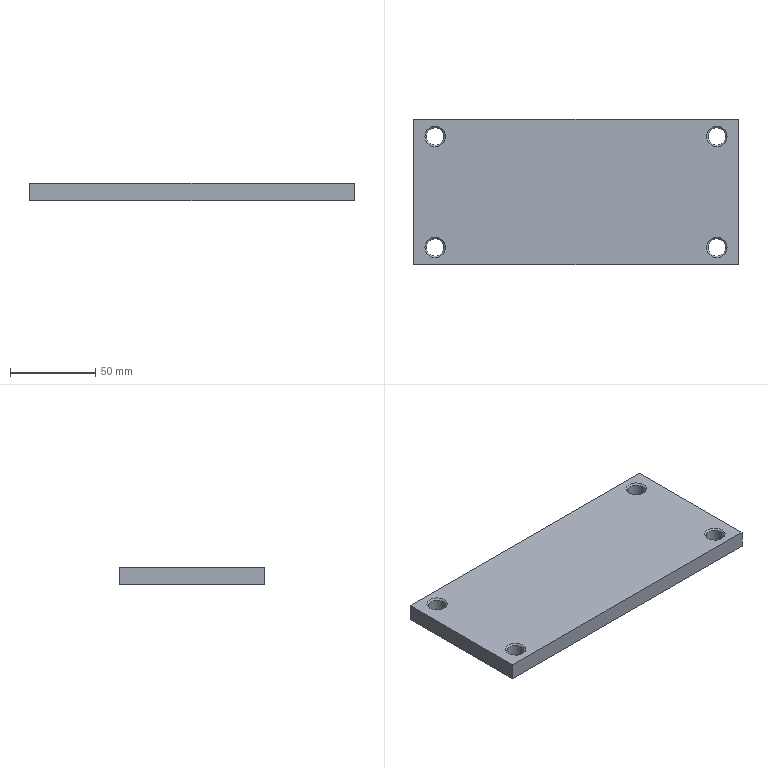Part | STEP file | Plate | 1 solid | 22 faces | box 190 x 85 x 10 mm | volume 158173 mm3 | cone 8 | cylinder 8 | plane 6 | commonest cylinder face diameters 10.2 x8
STEP:
#1=CARTESIAN_POINT('',(-147.6,57.5,9.075));
#2=VERTEX_POINT('',#1);
#3=CARTESIAN_POINT('',(-137.4,57.5,9.075));
#4=VERTEX_POINT('',#3);
#5=CARTESIAN_POINT('',(-142.5,57.5,9.075));
#6=DIRECTION('',(0.,0.,1.));
#7=DIRECTION('',(1.,0.,0.));
#8=AXIS2_PLACEMENT_3D('',#5,#6,#7);
#9=CIRCLE('',#8,5.1);
#10=EDGE_CURVE('',#2,#4,#9,.T.);
#11=ORIENTED_EDGE('',*,*,#10,.F.);
#12=CARTESIAN_POINT('',(-148.525,57.5,10.));
#13=VERTEX_POINT('',#12);
#14=CARTESIAN_POINT('',(-148.525,57.5,10.));
#15=DIRECTION('',(-0.7071,0.,0.7071));
#16=VECTOR('',#15,1000.);
#17=LINE('',#14,#16);
#18=EDGE_CURVE('',#2,#13,#17,.T.);
#19=ORIENTED_EDGE('',*,*,#18,.T.);
#20=CARTESIAN_POINT('',(-136.475,57.5,10.));
#21=VERTEX_POINT('',#20);
#22=CARTESIAN_POINT('',(-142.5,57.5,10.));
#23=DIRECTION('',(0.,0.,1.));
#24=DIRECTION('',(1.,0.,0.));
#25=AXIS2_PLACEMENT_3D('',#22,#23,#24);
#26=CIRCLE('',#25,6.025);
#27=EDGE_CURVE('',#13,#21,#26,.T.);
#28=ORIENTED_EDGE('',*,*,#27,.T.);
#29=CARTESIAN_POINT('',(-136.475,57.5,10.));
#30=DIRECTION('',(0.7071,0.,0.7071));
#31=VECTOR('',#30,1000.);
#32=LINE('',#29,#31);
#33=EDGE_CURVE('',#4,#21,#32,.T.);
#34=ORIENTED_EDGE('',*,*,#33,.F.);
#35=EDGE_LOOP('',(#11,#19,#28,#34));
#36=FACE_OUTER_BOUND('',#35,.T.);
#37=CARTESIAN_POINT('',(-142.5,57.5,10.));
#38=DIRECTION('',(0.,0.,1.));
#39=DIRECTION('',(1.,0.,0.));
#40=AXIS2_PLACEMENT_3D('',#37,#38,#39);
#41=CONICAL_SURFACE('',#40,6.025,0.7854);
#42=ADVANCED_FACE('',(#36),#41,.F.);
#43=CARTESIAN_POINT('',(-137.4,57.5,0.));
#44=VERTEX_POINT('',#43);
#45=CARTESIAN_POINT('',(-147.6,57.5,0.));
#46=VERTEX_POINT('',#45);
#47=CARTESIAN_POINT('',(-142.5,57.5,0.));
#48=DIRECTION('',(0.,0.,-1.));
#49=DIRECTION('',(-1.,0.,0.));
#50=AXIS2_PLACEMENT_3D('',#47,#48,#49);
#51=CIRCLE('',#50,5.1);
#52=EDGE_CURVE('',#44,#46,#51,.T.);
#53=ORIENTED_EDGE('',*,*,#52,.T.);
#54=CARTESIAN_POINT('',(-147.6,57.5,10.));
#55=DIRECTION('',(0.,0.,1.));
#56=VECTOR('',#55,1000.);
#57=LINE('',#54,#56);
#58=EDGE_CURVE('',#46,#2,#57,.T.);
#59=ORIENTED_EDGE('',*,*,#58,.T.);
#60=ORIENTED_EDGE('',*,*,#10,.T.);
#61=CARTESIAN_POINT('',(-137.4,57.5,10.));
#62=DIRECTION('',(0.,0.,1.));
#63=VECTOR('',#62,1000.);
#64=LINE('',#61,#63);
#65=EDGE_CURVE('',#44,#4,#64,.T.);
#66=ORIENTED_EDGE('',*,*,#65,.F.);
#67=EDGE_LOOP('',(#53,#59,#60,#66));
#68=FACE_OUTER_BOUND('',#67,.T.);
#69=CARTESIAN_POINT('',(-142.5,57.5,10.));
#70=DIRECTION('',(0.,0.,1.));
#71=DIRECTION('',(1.,0.,0.));
#72=AXIS2_PLACEMENT_3D('',#69,#70,#71);
#73=CYLINDRICAL_SURFACE('',#72,5.1);
#74=ADVANCED_FACE('',(#68),#73,.F.);
#75=CARTESIAN_POINT('',(-147.6,-7.5,9.075));
#76=VERTEX_POINT('',#75);
#77=CARTESIAN_POINT('',(-137.4,-7.5,9.075));
#78=VERTEX_POINT('',#77);
#79=CARTESIAN_POINT('',(-142.5,-7.5,9.075));
#80=DIRECTION('',(0.,0.,1.));
#81=DIRECTION('',(1.,0.,0.));
#82=AXIS2_PLACEMENT_3D('',#79,#80,#81);
#83=CIRCLE('',#82,5.1);
#84=EDGE_CURVE('',#76,#78,#83,.T.);
#85=ORIENTED_EDGE('',*,*,#84,.F.);
#86=CARTESIAN_POINT('',(-148.525,-7.5,10.));
#87=VERTEX_POINT('',#86);
#88=CARTESIAN_POINT('',(-148.525,-7.5,10.));
#89=DIRECTION('',(-0.7071,0.,0.7071));
#90=VECTOR('',#89,1000.);
#91=LINE('',#88,#90);
#92=EDGE_CURVE('',#76,#87,#91,.T.);
#93=ORIENTED_EDGE('',*,*,#92,.T.);
#94=CARTESIAN_POINT('',(-136.475,-7.5,10.));
#95=VERTEX_POINT('',#94);
#96=CARTESIAN_POINT('',(-142.5,-7.5,10.));
#97=DIRECTION('',(0.,0.,1.));
#98=DIRECTION('',(1.,0.,0.));
#99=AXIS2_PLACEMENT_3D('',#96,#97,#98);
#100=CIRCLE('',#99,6.025);
#101=EDGE_CURVE('',#87,#95,#100,.T.);
#102=ORIENTED_EDGE('',*,*,#101,.T.);
#103=CARTESIAN_POINT('',(-136.475,-7.5,10.));
#104=DIRECTION('',(0.7071,0.,0.7071));
#105=VECTOR('',#104,1000.);
#106=LINE('',#103,#105);
#107=EDGE_CURVE('',#78,#95,#106,.T.);
#108=ORIENTED_EDGE('',*,*,#107,.F.);
#109=EDGE_LOOP('',(#85,#93,#102,#108));
#110=FACE_OUTER_BOUND('',#109,.T.);
#111=CARTESIAN_POINT('',(-142.5,-7.5,10.));
#112=DIRECTION('',(0.,0.,1.));
#113=DIRECTION('',(1.,0.,0.));
#114=AXIS2_PLACEMENT_3D('',#111,#112,#113);
#115=CONICAL_SURFACE('',#114,6.025,0.7854);
#116=ADVANCED_FACE('',(#110),#115,.F.);
#117=CARTESIAN_POINT('',(-137.4,-7.5,0.));
#118=VERTEX_POINT('',#117);
#119=CARTESIAN_POINT('',(-147.6,-7.5,0.));
#120=VERTEX_POINT('',#119);
#121=CARTESIAN_POINT('',(-142.5,-7.5,0.));
#122=DIRECTION('',(0.,0.,-1.));
#123=DIRECTION('',(-1.,0.,0.));
#124=AXIS2_PLACEMENT_3D('',#121,#122,#123);
#125=CIRCLE('',#124,5.1);
#126=EDGE_CURVE('',#118,#120,#125,.T.);
#127=ORIENTED_EDGE('',*,*,#126,.T.);
#128=CARTESIAN_POINT('',(-147.6,-7.5,10.));
#129=DIRECTION('',(0.,0.,1.));
#130=VECTOR('',#129,1000.);
#131=LINE('',#128,#130);
#132=EDGE_CURVE('',#120,#76,#131,.T.);
#133=ORIENTED_EDGE('',*,*,#132,.T.);
#134=ORIENTED_EDGE('',*,*,#84,.T.);
#135=CARTESIAN_POINT('',(-137.4,-7.5,10.));
#136=DIRECTION('',(0.,0.,1.));
#137=VECTOR('',#136,1000.);
#138=LINE('',#135,#137);
#139=EDGE_CURVE('',#118,#78,#138,.T.);
#140=ORIENTED_EDGE('',*,*,#139,.F.);
#141=EDGE_LOOP('',(#127,#133,#134,#140));
#142=FACE_OUTER_BOUND('',#141,.T.);
#143=CARTESIAN_POINT('',(-142.5,-7.5,10.));
#144=DIRECTION('',(0.,0.,1.));
#145=DIRECTION('',(1.,0.,0.));
#146=AXIS2_PLACEMENT_3D('',#143,#144,#145);
#147=CYLINDRICAL_SURFACE('',#146,5.1);
#148=ADVANCED_FACE('',(#142),#147,.F.);
#149=CARTESIAN_POINT('',(17.4,-7.5,9.075));
#150=VERTEX_POINT('',#149);
#151=CARTESIAN_POINT('',(27.6,-7.5,9.075));
#152=VERTEX_POINT('',#151);
#153=CARTESIAN_POINT('',(22.5,-7.5,9.075));
#154=DIRECTION('',(0.,0.,1.));
#155=DIRECTION('',(1.,0.,0.));
#156=AXIS2_PLACEMENT_3D('',#153,#154,#155);
#157=CIRCLE('',#156,5.1);
#158=EDGE_CURVE('',#150,#152,#157,.T.);
#159=ORIENTED_EDGE('',*,*,#158,.F.);
#160=CARTESIAN_POINT('',(16.475,-7.5,10.));
#161=VERTEX_POINT('',#160);
#162=CARTESIAN_POINT('',(16.475,-7.5,10.));
#163=DIRECTION('',(-0.7071,0.,0.7071));
#164=VECTOR('',#163,1000.);
#165=LINE('',#162,#164);
#166=EDGE_CURVE('',#150,#161,#165,.T.);
#167=ORIENTED_EDGE('',*,*,#166,.T.);
#168=CARTESIAN_POINT('',(28.525,-7.5,10.));
#169=VERTEX_POINT('',#168);
#170=CARTESIAN_POINT('',(22.5,-7.5,10.));
#171=DIRECTION('',(0.,0.,1.));
#172=DIRECTION('',(1.,0.,0.));
#173=AXIS2_PLACEMENT_3D('',#170,#171,#172);
#174=CIRCLE('',#173,6.025);
#175=EDGE_CURVE('',#161,#169,#174,.T.);
#176=ORIENTED_EDGE('',*,*,#175,.T.);
#177=CARTESIAN_POINT('',(28.525,-7.5,10.));
#178=DIRECTION('',(0.7071,0.,0.7071));
#179=VECTOR('',#178,1000.);
#180=LINE('',#177,#179);
#181=EDGE_CURVE('',#152,#169,#180,.T.);
#182=ORIENTED_EDGE('',*,*,#181,.F.);
#183=EDGE_LOOP('',(#159,#167,#176,#182));
#184=FACE_OUTER_BOUND('',#183,.T.);
#185=CARTESIAN_POINT('',(22.5,-7.5,10.));
#186=DIRECTION('',(0.,0.,1.));
#187=DIRECTION('',(1.,0.,0.));
#188=AXIS2_PLACEMENT_3D('',#185,#186,#187);
#189=CONICAL_SURFACE('',#188,6.025,0.7854);
#190=ADVANCED_FACE('',(#184),#189,.F.);
#191=CARTESIAN_POINT('',(27.6,-7.5,0.));
#192=VERTEX_POINT('',#191);
#193=CARTESIAN_POINT('',(17.4,-7.5,0.));
#194=VERTEX_POINT('',#193);
#195=CARTESIAN_POINT('',(22.5,-7.5,0.));
#196=DIRECTION('',(0.,0.,-1.));
#197=DIRECTION('',(-1.,0.,0.));
#198=AXIS2_PLACEMENT_3D('',#195,#196,#197);
#199=CIRCLE('',#198,5.1);
#200=EDGE_CURVE('',#192,#194,#199,.T.);
#201=ORIENTED_EDGE('',*,*,#200,.T.);
#202=CARTESIAN_POINT('',(17.4,-7.5,10.));
#203=DIRECTION('',(0.,0.,1.));
#204=VECTOR('',#203,1000.);
#205=LINE('',#202,#204);
#206=EDGE_CURVE('',#194,#150,#205,.T.);
#207=ORIENTED_EDGE('',*,*,#206,.T.);
#208=ORIENTED_EDGE('',*,*,#158,.T.);
#209=CARTESIAN_POINT('',(27.6,-7.5,10.));
#210=DIRECTION('',(0.,0.,1.));
#211=VECTOR('',#210,1000.);
#212=LINE('',#209,#211);
#213=EDGE_CURVE('',#192,#152,#212,.T.);
#214=ORIENTED_EDGE('',*,*,#213,.F.);
#215=EDGE_LOOP('',(#201,#207,#208,#214));
#216=FACE_OUTER_BOUND('',#215,.T.);
#217=CARTESIAN_POINT('',(22.5,-7.5,10.));
#218=DIRECTION('',(0.,0.,1.));
#219=DIRECTION('',(1.,0.,0.));
#220=AXIS2_PLACEMENT_3D('',#217,#218,#219);
#221=CYLINDRICAL_SURFACE('',#220,5.1);
#222=ADVANCED_FACE('',(#216),#221,.F.);
#223=CARTESIAN_POINT('',(17.4,57.5,9.075));
#224=VERTEX_POINT('',#223);
#225=CARTESIAN_POINT('',(27.6,57.5,9.075));
#226=VERTEX_POINT('',#225);
#227=CARTESIAN_POINT('',(22.5,57.5,9.075));
#228=DIRECTION('',(0.,0.,1.));
#229=DIRECTION('',(1.,0.,0.));
#230=AXIS2_PLACEMENT_3D('',#227,#228,#229);
#231=CIRCLE('',#230,5.1);
#232=EDGE_CURVE('',#224,#226,#231,.T.);
#233=ORIENTED_EDGE('',*,*,#232,.F.);
#234=CARTESIAN_POINT('',(16.475,57.5,10.));
#235=VERTEX_POINT('',#234);
#236=CARTESIAN_POINT('',(16.475,57.5,10.));
#237=DIRECTION('',(-0.7071,0.,0.7071));
#238=VECTOR('',#237,1000.);
#239=LINE('',#236,#238);
#240=EDGE_CURVE('',#224,#235,#239,.T.);
#241=ORIENTED_EDGE('',*,*,#240,.T.);
#242=CARTESIAN_POINT('',(28.525,57.5,10.));
#243=VERTEX_POINT('',#242);
#244=CARTESIAN_POINT('',(22.5,57.5,10.));
#245=DIRECTION('',(0.,0.,1.));
#246=DIRECTION('',(1.,0.,0.));
#247=AXIS2_PLACEMENT_3D('',#244,#245,#246);
#248=CIRCLE('',#247,6.025);
#249=EDGE_CURVE('',#235,#243,#248,.T.);
#250=ORIENTED_EDGE('',*,*,#249,.T.);
#251=CARTESIAN_POINT('',(28.525,57.5,10.));
#252=DIRECTION('',(0.7071,0.,0.7071));
#253=VECTOR('',#252,1000.);
#254=LINE('',#251,#253);
#255=EDGE_CURVE('',#226,#243,#254,.T.);
#256=ORIENTED_EDGE('',*,*,#255,.F.);
#257=EDGE_LOOP('',(#233,#241,#250,#256));
#258=FACE_OUTER_BOUND('',#257,.T.);
#259=CARTESIAN_POINT('',(22.5,57.5,10.));
#260=DIRECTION('',(0.,0.,1.));
#261=DIRECTION('',(1.,0.,0.));
#262=AXIS2_PLACEMENT_3D('',#259,#260,#261);
#263=CONICAL_SURFACE('',#262,6.025,0.7854);
#264=ADVANCED_FACE('',(#258),#263,.F.);
#265=CARTESIAN_POINT('',(27.6,57.5,0.));
#266=VERTEX_POINT('',#265);
#267=CARTESIAN_POINT('',(17.4,57.5,0.));
#268=VERTEX_POINT('',#267);
#269=CARTESIAN_POINT('',(22.5,57.5,0.));
#270=DIRECTION('',(0.,0.,-1.));
#271=DIRECTION('',(-1.,0.,0.));
#272=AXIS2_PLACEMENT_3D('',#269,#270,#271);
#273=CIRCLE('',#272,5.1);
#274=EDGE_CURVE('',#266,#268,#273,.T.);
#275=ORIENTED_EDGE('',*,*,#274,.T.);
#276=CARTESIAN_POINT('',(17.4,57.5,10.));
#277=DIRECTION('',(0.,0.,1.));
#278=VECTOR('',#277,1000.);
#279=LINE('',#276,#278);
#280=EDGE_CURVE('',#268,#224,#279,.T.);
#281=ORIENTED_EDGE('',*,*,#280,.T.);
#282=ORIENTED_EDGE('',*,*,#232,.T.);
#283=CARTESIAN_POINT('',(27.6,57.5,10.));
#284=DIRECTION('',(0.,0.,1.));
#285=VECTOR('',#284,1000.);
#286=LINE('',#283,#285);
#287=EDGE_CURVE('',#266,#226,#286,.T.);
#288=ORIENTED_EDGE('',*,*,#287,.F.);
#289=EDGE_LOOP('',(#275,#281,#282,#288));
#290=FACE_OUTER_BOUND('',#289,.T.);
#291=CARTESIAN_POINT('',(22.5,57.5,10.));
#292=DIRECTION('',(0.,0.,1.));
#293=DIRECTION('',(1.,0.,0.));
#294=AXIS2_PLACEMENT_3D('',#291,#292,#293);
#295=CYLINDRICAL_SURFACE('',#294,5.1);
#296=ADVANCED_FACE('',(#290),#295,.F.);
#297=CARTESIAN_POINT('',(-155.,67.5,10.));
#298=VERTEX_POINT('',#297);
#299=CARTESIAN_POINT('',(-155.,-17.5,10.));
#300=VERTEX_POINT('',#299);
#301=CARTESIAN_POINT('',(-155.,67.5,10.));
#302=DIRECTION('',(0.,-1.,0.));
#303=VECTOR('',#302,1000.);
#304=LINE('',#301,#303);
#305=EDGE_CURVE('',#298,#300,#304,.T.);
#306=ORIENTED_EDGE('',*,*,#305,.T.);
#307=CARTESIAN_POINT('',(35.,-17.5,10.));
#308=VERTEX_POINT('',#307);
#309=CARTESIAN_POINT('',(35.,-17.5,10.));
#310=DIRECTION('',(1.,0.,0.));
#311=VECTOR('',#310,1000.);
#312=LINE('',#309,#311);
#313=EDGE_CURVE('',#300,#308,#312,.T.);
#314=ORIENTED_EDGE('',*,*,#313,.T.);
#315=CARTESIAN_POINT('',(35.,67.5,10.));
#316=VERTEX_POINT('',#315);
#317=CARTESIAN_POINT('',(35.,67.5,10.));
#318=DIRECTION('',(0.,1.,0.));
#319=VECTOR('',#318,1000.);
#320=LINE('',#317,#319);
#321=EDGE_CURVE('',#308,#316,#320,.T.);
#322=ORIENTED_EDGE('',*,*,#321,.T.);
#323=CARTESIAN_POINT('',(35.,67.5,10.));
#324=DIRECTION('',(-1.,0.,0.));
#325=VECTOR('',#324,1000.);
#326=LINE('',#323,#325);
#327=EDGE_CURVE('',#316,#298,#326,.T.);
#328=ORIENTED_EDGE('',*,*,#327,.T.);
#329=EDGE_LOOP('',(#306,#314,#322,#328));
#330=FACE_OUTER_BOUND('',#329,.T.);
#331=CARTESIAN_POINT('',(22.5,57.5,10.));
#332=DIRECTION('',(0.,0.,1.));
#333=DIRECTION('',(1.,0.,0.));
#334=AXIS2_PLACEMENT_3D('',#331,#332,#333);
#335=CIRCLE('',#334,6.025);
#336=EDGE_CURVE('',#243,#235,#335,.T.);
#337=ORIENTED_EDGE('',*,*,#336,.F.);
#338=ORIENTED_EDGE('',*,*,#249,.F.);
#339=EDGE_LOOP('',(#337,#338));
#340=FACE_BOUND('',#339,.T.);
#341=CARTESIAN_POINT('',(22.5,-7.5,10.));
#342=DIRECTION('',(0.,0.,1.));
#343=DIRECTION('',(1.,0.,0.));
#344=AXIS2_PLACEMENT_3D('',#341,#342,#343);
#345=CIRCLE('',#344,6.025);
#346=EDGE_CURVE('',#169,#161,#345,.T.);
#347=ORIENTED_EDGE('',*,*,#346,.F.);
#348=ORIENTED_EDGE('',*,*,#175,.F.);
#349=EDGE_LOOP('',(#347,#348));
#350=FACE_BOUND('',#349,.T.);
#351=CARTESIAN_POINT('',(-142.5,-7.5,10.));
#352=DIRECTION('',(0.,0.,1.));
#353=DIRECTION('',(1.,0.,0.));
#354=AXIS2_PLACEMENT_3D('',#351,#352,#353);
#355=CIRCLE('',#354,6.025);
#356=EDGE_CURVE('',#95,#87,#355,.T.);
#357=ORIENTED_EDGE('',*,*,#356,.F.);
#358=ORIENTED_EDGE('',*,*,#101,.F.);
#359=EDGE_LOOP('',(#357,#358));
#360=FACE_BOUND('',#359,.T.);
#361=CARTESIAN_POINT('',(-142.5,57.5,10.));
#362=DIRECTION('',(0.,0.,1.));
#363=DIRECTION('',(1.,0.,0.));
#364=AXIS2_PLACEMENT_3D('',#361,#362,#363);
#365=CIRCLE('',#364,6.025);
#366=EDGE_CURVE('',#21,#13,#365,.T.);
#367=ORIENTED_EDGE('',*,*,#366,.F.);
#368=ORIENTED_EDGE('',*,*,#27,.F.);
#369=EDGE_LOOP('',(#367,#368));
#370=FACE_BOUND('',#369,.T.);
#371=CARTESIAN_POINT('',(0.,0.,10.));
#372=DIRECTION('',(0.,0.,-1.));
#373=DIRECTION('',(-1.,0.,0.));
#374=AXIS2_PLACEMENT_3D('',#371,#372,#373);
#375=PLANE('',#374);
#376=ADVANCED_FACE('',(#330,#340,#350,#360,#370),#375,.F.);
#377=CARTESIAN_POINT('',(-155.,67.5,0.));
#378=VERTEX_POINT('',#377);
#379=CARTESIAN_POINT('',(-155.,-17.5,0.));
#380=VERTEX_POINT('',#379);
#381=CARTESIAN_POINT('',(-155.,67.5,0.));
#382=DIRECTION('',(0.,-1.,0.));
#383=VECTOR('',#382,1000.);
#384=LINE('',#381,#383);
#385=EDGE_CURVE('',#378,#380,#384,.T.);
#386=ORIENTED_EDGE('',*,*,#385,.T.);
#387=CARTESIAN_POINT('',(-155.,-17.5,10.));
#388=DIRECTION('',(0.,0.,-1.));
#389=VECTOR('',#388,1000.);
#390=LINE('',#387,#389);
#391=EDGE_CURVE('',#300,#380,#390,.T.);
#392=ORIENTED_EDGE('',*,*,#391,.F.);
#393=ORIENTED_EDGE('',*,*,#305,.F.);
#394=CARTESIAN_POINT('',(-155.,67.5,10.));
#395=DIRECTION('',(0.,0.,-1.));
#396=VECTOR('',#395,1000.);
#397=LINE('',#394,#396);
#398=EDGE_CURVE('',#298,#378,#397,.T.);
#399=ORIENTED_EDGE('',*,*,#398,.T.);
#400=EDGE_LOOP('',(#386,#392,#393,#399));
#401=FACE_OUTER_BOUND('',#400,.T.);
#402=CARTESIAN_POINT('',(-155.,67.5,10.));
#403=DIRECTION('',(1.,0.,0.));
#404=DIRECTION('',(0.,0.,-1.));
#405=AXIS2_PLACEMENT_3D('',#402,#403,#404);
#406=PLANE('',#405);
#407=ADVANCED_FACE('',(#401),#406,.F.);
#408=CARTESIAN_POINT('',(35.,-17.5,0.));
#409=VERTEX_POINT('',#408);
#410=CARTESIAN_POINT('',(35.,-17.5,0.));
#411=DIRECTION('',(1.,0.,0.));
#412=VECTOR('',#411,1000.);
#413=LINE('',#410,#412);
#414=EDGE_CURVE('',#380,#409,#413,.T.);
#415=ORIENTED_EDGE('',*,*,#414,.T.);
#416=CARTESIAN_POINT('',(35.,-17.5,10.));
#417=DIRECTION('',(0.,0.,-1.));
#418=VECTOR('',#417,1000.);
#419=LINE('',#416,#418);
#420=EDGE_CURVE('',#308,#409,#419,.T.);
#421=ORIENTED_EDGE('',*,*,#420,.F.);
#422=ORIENTED_EDGE('',*,*,#313,.F.);
#423=ORIENTED_EDGE('',*,*,#391,.T.);
#424=EDGE_LOOP('',(#415,#421,#422,#423));
#425=FACE_OUTER_BOUND('',#424,.T.);
#426=CARTESIAN_POINT('',(35.,-17.5,10.));
#427=DIRECTION('',(0.,1.,0.));
#428=DIRECTION('',(-1.,0.,0.));
#429=AXIS2_PLACEMENT_3D('',#426,#427,#428);
#430=PLANE('',#429);
#431=ADVANCED_FACE('',(#425),#430,.F.);
#432=CARTESIAN_POINT('',(35.,67.5,0.));
#433=VERTEX_POINT('',#432);
#434=CARTESIAN_POINT('',(35.,67.5,0.));
#435=DIRECTION('',(0.,1.,0.));
#436=VECTOR('',#435,1000.);
#437=LINE('',#434,#436);
#438=EDGE_CURVE('',#409,#433,#437,.T.);
#439=ORIENTED_EDGE('',*,*,#438,.T.);
#440=CARTESIAN_POINT('',(35.,67.5,10.));
#441=DIRECTION('',(0.,0.,-1.));
#442=VECTOR('',#441,1000.);
#443=LINE('',#440,#442);
#444=EDGE_CURVE('',#316,#433,#443,.T.);
#445=ORIENTED_EDGE('',*,*,#444,.F.);
#446=ORIENTED_EDGE('',*,*,#321,.F.);
#447=ORIENTED_EDGE('',*,*,#420,.T.);
#448=EDGE_LOOP('',(#439,#445,#446,#447));
#449=FACE_OUTER_BOUND('',#448,.T.);
#450=CARTESIAN_POINT('',(35.,67.5,10.));
#451=DIRECTION('',(-1.,0.,0.));
#452=DIRECTION('',(0.,0.,1.));
#453=AXIS2_PLACEMENT_3D('',#450,#451,#452);
#454=PLANE('',#453);
#455=ADVANCED_FACE('',(#449),#454,.F.);
#456=CARTESIAN_POINT('',(35.,67.5,0.));
#457=DIRECTION('',(-1.,0.,0.));
#458=VECTOR('',#457,1000.);
#459=LINE('',#456,#458);
#460=EDGE_CURVE('',#433,#378,#459,.T.);
#461=ORIENTED_EDGE('',*,*,#460,.T.);
#462=ORIENTED_EDGE('',*,*,#398,.F.);
#463=ORIENTED_EDGE('',*,*,#327,.F.);
#464=ORIENTED_EDGE('',*,*,#444,.T.);
#465=EDGE_LOOP('',(#461,#462,#463,#464));
#466=FACE_OUTER_BOUND('',#465,.T.);
#467=CARTESIAN_POINT('',(35.,67.5,10.));
#468=DIRECTION('',(0.,-1.,0.));
#469=DIRECTION('',(1.,0.,0.));
#470=AXIS2_PLACEMENT_3D('',#467,#468,#469);
#471=PLANE('',#470);
#472=ADVANCED_FACE('',(#466),#471,.F.);
#473=ORIENTED_EDGE('',*,*,#52,.F.);
#474=CARTESIAN_POINT('',(-142.5,57.5,0.));
#475=DIRECTION('',(0.,0.,-1.));
#476=DIRECTION('',(-1.,0.,0.));
#477=AXIS2_PLACEMENT_3D('',#474,#475,#476);
#478=CIRCLE('',#477,5.1);
#479=EDGE_CURVE('',#46,#44,#478,.T.);
#480=ORIENTED_EDGE('',*,*,#479,.F.);
#481=EDGE_LOOP('',(#473,#480));
#482=FACE_BOUND('',#481,.T.);
#483=ORIENTED_EDGE('',*,*,#126,.F.);
#484=CARTESIAN_POINT('',(-142.5,-7.5,0.));
#485=DIRECTION('',(0.,0.,-1.));
#486=DIRECTION('',(-1.,0.,0.));
#487=AXIS2_PLACEMENT_3D('',#484,#485,#486);
#488=CIRCLE('',#487,5.1);
#489=EDGE_CURVE('',#120,#118,#488,.T.);
#490=ORIENTED_EDGE('',*,*,#489,.F.);
#491=EDGE_LOOP('',(#483,#490));
#492=FACE_BOUND('',#491,.T.);
#493=ORIENTED_EDGE('',*,*,#200,.F.);
#494=CARTESIAN_POINT('',(22.5,-7.5,0.));
#495=DIRECTION('',(0.,0.,-1.));
#496=DIRECTION('',(-1.,0.,0.));
#497=AXIS2_PLACEMENT_3D('',#494,#495,#496);
#498=CIRCLE('',#497,5.1);
#499=EDGE_CURVE('',#194,#192,#498,.T.);
#500=ORIENTED_EDGE('',*,*,#499,.F.);
#501=EDGE_LOOP('',(#493,#500));
#502=FACE_BOUND('',#501,.T.);
#503=ORIENTED_EDGE('',*,*,#274,.F.);
#504=CARTESIAN_POINT('',(22.5,57.5,0.));
#505=DIRECTION('',(0.,0.,-1.));
#506=DIRECTION('',(-1.,0.,0.));
#507=AXIS2_PLACEMENT_3D('',#504,#505,#506);
#508=CIRCLE('',#507,5.1);
#509=EDGE_CURVE('',#268,#266,#508,.T.);
#510=ORIENTED_EDGE('',*,*,#509,.F.);
#511=EDGE_LOOP('',(#503,#510));
#512=FACE_BOUND('',#511,.T.);
#513=ORIENTED_EDGE('',*,*,#385,.F.);
#514=ORIENTED_EDGE('',*,*,#460,.F.);
#515=ORIENTED_EDGE('',*,*,#438,.F.);
#516=ORIENTED_EDGE('',*,*,#414,.F.);
#517=EDGE_LOOP('',(#513,#514,#515,#516));
#518=FACE_OUTER_BOUND('',#517,.T.);
#519=CARTESIAN_POINT('',(0.,0.,0.));
#520=DIRECTION('',(0.,0.,-1.));
#521=DIRECTION('',(-1.,0.,0.));
#522=AXIS2_PLACEMENT_3D('',#519,#520,#521);
#523=PLANE('',#522);
#524=ADVANCED_FACE('',(#482,#492,#502,#512,#518),#523,.T.);
#525=ORIENTED_EDGE('',*,*,#280,.F.);
#526=ORIENTED_EDGE('',*,*,#509,.T.);
#527=ORIENTED_EDGE('',*,*,#287,.T.);
#528=CARTESIAN_POINT('',(22.5,57.5,9.075));
#529=DIRECTION('',(0.,0.,1.));
#530=DIRECTION('',(1.,0.,0.));
#531=AXIS2_PLACEMENT_3D('',#528,#529,#530);
#532=CIRCLE('',#531,5.1);
#533=EDGE_CURVE('',#226,#224,#532,.T.);
#534=ORIENTED_EDGE('',*,*,#533,.T.);
#535=EDGE_LOOP('',(#525,#526,#527,#534));
#536=FACE_OUTER_BOUND('',#535,.T.);
#537=CARTESIAN_POINT('',(22.5,57.5,10.));
#538=DIRECTION('',(0.,0.,1.));
#539=DIRECTION('',(1.,0.,0.));
#540=AXIS2_PLACEMENT_3D('',#537,#538,#539);
#541=CYLINDRICAL_SURFACE('',#540,5.1);
#542=ADVANCED_FACE('',(#536),#541,.F.);
#543=ORIENTED_EDGE('',*,*,#240,.F.);
#544=ORIENTED_EDGE('',*,*,#533,.F.);
#545=ORIENTED_EDGE('',*,*,#255,.T.);
#546=ORIENTED_EDGE('',*,*,#336,.T.);
#547=EDGE_LOOP('',(#543,#544,#545,#546));
#548=FACE_OUTER_BOUND('',#547,.T.);
#549=CARTESIAN_POINT('',(22.5,57.5,10.));
#550=DIRECTION('',(0.,0.,1.));
#551=DIRECTION('',(1.,0.,0.));
#552=AXIS2_PLACEMENT_3D('',#549,#550,#551);
#553=CONICAL_SURFACE('',#552,6.025,0.7854);
#554=ADVANCED_FACE('',(#548),#553,.F.);
#555=ORIENTED_EDGE('',*,*,#206,.F.);
#556=ORIENTED_EDGE('',*,*,#499,.T.);
#557=ORIENTED_EDGE('',*,*,#213,.T.);
#558=CARTESIAN_POINT('',(22.5,-7.5,9.075));
#559=DIRECTION('',(0.,0.,1.));
#560=DIRECTION('',(1.,0.,0.));
#561=AXIS2_PLACEMENT_3D('',#558,#559,#560);
#562=CIRCLE('',#561,5.1);
#563=EDGE_CURVE('',#152,#150,#562,.T.);
#564=ORIENTED_EDGE('',*,*,#563,.T.);
#565=EDGE_LOOP('',(#555,#556,#557,#564));
#566=FACE_OUTER_BOUND('',#565,.T.);
#567=CARTESIAN_POINT('',(22.5,-7.5,10.));
#568=DIRECTION('',(0.,0.,1.));
#569=DIRECTION('',(1.,0.,0.));
#570=AXIS2_PLACEMENT_3D('',#567,#568,#569);
#571=CYLINDRICAL_SURFACE('',#570,5.1);
#572=ADVANCED_FACE('',(#566),#571,.F.);
#573=ORIENTED_EDGE('',*,*,#166,.F.);
#574=ORIENTED_EDGE('',*,*,#563,.F.);
#575=ORIENTED_EDGE('',*,*,#181,.T.);
#576=ORIENTED_EDGE('',*,*,#346,.T.);
#577=EDGE_LOOP('',(#573,#574,#575,#576));
#578=FACE_OUTER_BOUND('',#577,.T.);
#579=CARTESIAN_POINT('',(22.5,-7.5,10.));
#580=DIRECTION('',(0.,0.,1.));
#581=DIRECTION('',(1.,0.,0.));
#582=AXIS2_PLACEMENT_3D('',#579,#580,#581);
#583=CONICAL_SURFACE('',#582,6.025,0.7854);
#584=ADVANCED_FACE('',(#578),#583,.F.);
#585=ORIENTED_EDGE('',*,*,#132,.F.);
#586=ORIENTED_EDGE('',*,*,#489,.T.);
#587=ORIENTED_EDGE('',*,*,#139,.T.);
#588=CARTESIAN_POINT('',(-142.5,-7.5,9.075));
#589=DIRECTION('',(0.,0.,1.));
#590=DIRECTION('',(1.,0.,0.));
#591=AXIS2_PLACEMENT_3D('',#588,#589,#590);
#592=CIRCLE('',#591,5.1);
#593=EDGE_CURVE('',#78,#76,#592,.T.);
#594=ORIENTED_EDGE('',*,*,#593,.T.);
#595=EDGE_LOOP('',(#585,#586,#587,#594));
#596=FACE_OUTER_BOUND('',#595,.T.);
#597=CARTESIAN_POINT('',(-142.5,-7.5,10.));
#598=DIRECTION('',(0.,0.,1.));
#599=DIRECTION('',(1.,0.,0.));
#600=AXIS2_PLACEMENT_3D('',#597,#598,#599);
#601=CYLINDRICAL_SURFACE('',#600,5.1);
#602=ADVANCED_FACE('',(#596),#601,.F.);
#603=ORIENTED_EDGE('',*,*,#92,.F.);
#604=ORIENTED_EDGE('',*,*,#593,.F.);
#605=ORIENTED_EDGE('',*,*,#107,.T.);
#606=ORIENTED_EDGE('',*,*,#356,.T.);
#607=EDGE_LOOP('',(#603,#604,#605,#606));
#608=FACE_OUTER_BOUND('',#607,.T.);
#609=CARTESIAN_POINT('',(-142.5,-7.5,10.));
#610=DIRECTION('',(0.,0.,1.));
#611=DIRECTION('',(1.,0.,0.));
#612=AXIS2_PLACEMENT_3D('',#609,#610,#611);
#613=CONICAL_SURFACE('',#612,6.025,0.7854);
#614=ADVANCED_FACE('',(#608),#613,.F.);
#615=ORIENTED_EDGE('',*,*,#58,.F.);
#616=ORIENTED_EDGE('',*,*,#479,.T.);
#617=ORIENTED_EDGE('',*,*,#65,.T.);
#618=CARTESIAN_POINT('',(-142.5,57.5,9.075));
#619=DIRECTION('',(0.,0.,1.));
#620=DIRECTION('',(1.,0.,0.));
#621=AXIS2_PLACEMENT_3D('',#618,#619,#620);
#622=CIRCLE('',#621,5.1);
#623=EDGE_CURVE('',#4,#2,#622,.T.);
#624=ORIENTED_EDGE('',*,*,#623,.T.);
#625=EDGE_LOOP('',(#615,#616,#617,#624));
#626=FACE_OUTER_BOUND('',#625,.T.);
#627=CARTESIAN_POINT('',(-142.5,57.5,10.));
#628=DIRECTION('',(0.,0.,1.));
#629=DIRECTION('',(1.,0.,0.));
#630=AXIS2_PLACEMENT_3D('',#627,#628,#629);
#631=CYLINDRICAL_SURFACE('',#630,5.1);
#632=ADVANCED_FACE('',(#626),#631,.F.);
#633=ORIENTED_EDGE('',*,*,#18,.F.);
#634=ORIENTED_EDGE('',*,*,#623,.F.);
#635=ORIENTED_EDGE('',*,*,#33,.T.);
#636=ORIENTED_EDGE('',*,*,#366,.T.);
#637=EDGE_LOOP('',(#633,#634,#635,#636));
#638=FACE_OUTER_BOUND('',#637,.T.);
#639=CARTESIAN_POINT('',(-142.5,57.5,10.));
#640=DIRECTION('',(0.,0.,1.));
#641=DIRECTION('',(1.,0.,0.));
#642=AXIS2_PLACEMENT_3D('',#639,#640,#641);
#643=CONICAL_SURFACE('',#642,6.025,0.7854);
#644=ADVANCED_FACE('',(#638),#643,.F.);
#645=CLOSED_SHELL('',(#42,#74,#116,#148,#190,#222,#264,#296,#376,#407,#431,#455,#472,#524,#542,#554,#572,#584,#602,#614,#632,#644));
#646=MANIFOLD_SOLID_BREP('',#645);
#647=CARTESIAN_POINT('',(0.,0.,0.));
#648=DIRECTION('',(0.,0.,1.));
#649=DIRECTION('',(1.,0.,0.));
#650=AXIS2_PLACEMENT_3D('',#647,#648,#649);
#651=(LENGTH_UNIT()NAMED_UNIT(*)SI_UNIT(.MILLI.,.METRE.));
#652=UNCERTAINTY_MEASURE_WITH_UNIT(LENGTH_MEASURE(0.00001),#651,'','');
#653=(NAMED_UNIT(*)PLANE_ANGLE_UNIT()SI_UNIT($,.RADIAN.));
#654=(NAMED_UNIT(*)SI_UNIT($,.STERADIAN.)SOLID_ANGLE_UNIT());
#655=(GEOMETRIC_REPRESENTATION_CONTEXT(3)GLOBAL_UNCERTAINTY_ASSIGNED_CONTEXT((#652))GLOBAL_UNIT_ASSIGNED_CONTEXT((#651,#653,#654))REPRESENTATION_CONTEXT('',''));
#656=ADVANCED_BREP_SHAPE_REPRESENTATION('',(#646,#650),#655);